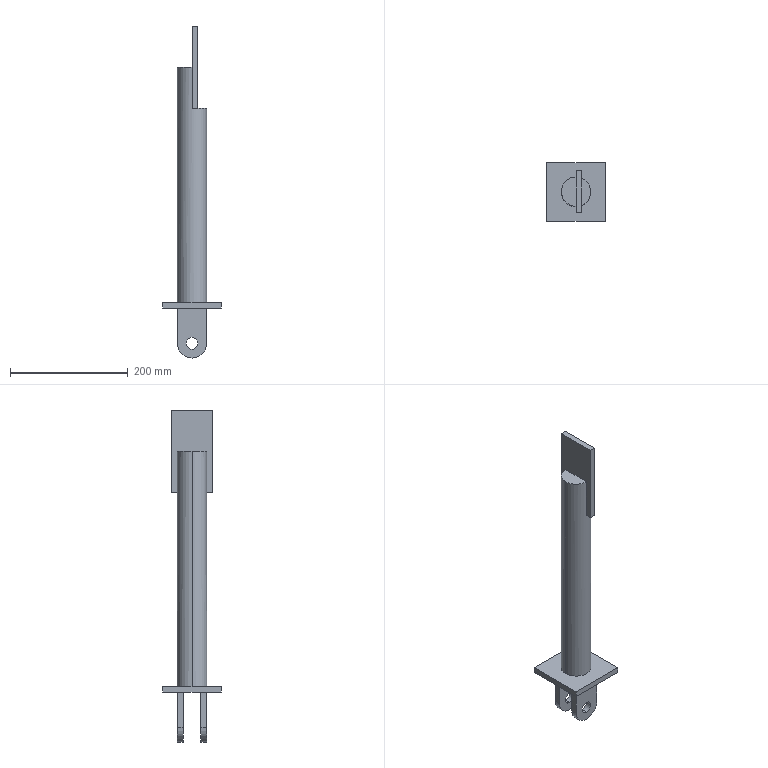Part | SolidWorks | features ICE 5, Extrusion 1 | 1 solid | 33 faces | box 100 x 100 x 565 mm | volume 988028 mm3 | plane 23 | cylinder 10 | commonest cylinder face diameters 50 x6 20 x4
STEP:
#1=CARTESIAN_POINT('',(25.,0.,335.));
#2=VERTEX_POINT('',#1);
#3=CARTESIAN_POINT('',(10.,22.913,335.));
#4=VERTEX_POINT('',#3);
#5=CARTESIAN_POINT('',(0.,0.,335.));
#6=DIRECTION('',(0.,0.,1.));
#7=DIRECTION('',(1.,0.,0.));
#8=AXIS2_PLACEMENT_3D('',#5,#6,#7);
#9=CIRCLE('',#8,25.);
#10=EDGE_CURVE('',#2,#4,#9,.T.);
#11=ORIENTED_EDGE('',*,*,#10,.F.);
#12=CARTESIAN_POINT('',(25.,0.,5.));
#13=VERTEX_POINT('',#12);
#14=CARTESIAN_POINT('',(25.,0.,405.));
#15=DIRECTION('',(0.,0.,-1.));
#16=VECTOR('',#15,1000.);
#17=LINE('',#14,#16);
#18=EDGE_CURVE('',#2,#13,#17,.T.);
#19=ORIENTED_EDGE('',*,*,#18,.T.);
#20=CARTESIAN_POINT('',(-25.,0.,5.));
#21=VERTEX_POINT('',#20);
#22=CARTESIAN_POINT('',(0.,0.,5.));
#23=DIRECTION('',(0.,0.,1.));
#24=DIRECTION('',(1.,0.,0.));
#25=AXIS2_PLACEMENT_3D('',#22,#23,#24);
#26=CIRCLE('',#25,25.);
#27=EDGE_CURVE('',#13,#21,#26,.T.);
#28=ORIENTED_EDGE('',*,*,#27,.T.);
#29=CARTESIAN_POINT('',(-25.,0.,405.));
#30=VERTEX_POINT('',#29);
#31=CARTESIAN_POINT('',(-25.,0.,405.));
#32=DIRECTION('',(0.,0.,-1.));
#33=VECTOR('',#32,1000.);
#34=LINE('',#31,#33);
#35=EDGE_CURVE('',#30,#21,#34,.T.);
#36=ORIENTED_EDGE('',*,*,#35,.F.);
#37=CARTESIAN_POINT('',(0.,25.,405.));
#38=VERTEX_POINT('',#37);
#39=CARTESIAN_POINT('',(0.,0.,405.));
#40=DIRECTION('',(0.,0.,1.));
#41=DIRECTION('',(1.,0.,0.));
#42=AXIS2_PLACEMENT_3D('',#39,#40,#41);
#43=CIRCLE('',#42,25.);
#44=EDGE_CURVE('',#38,#30,#43,.T.);
#45=ORIENTED_EDGE('',*,*,#44,.F.);
#46=CARTESIAN_POINT('',(0.,25.,335.));
#47=VERTEX_POINT('',#46);
#48=CARTESIAN_POINT('',(0.,25.,335.));
#49=DIRECTION('',(0.,0.,1.));
#50=VECTOR('',#49,1000.);
#51=LINE('',#48,#50);
#52=EDGE_CURVE('',#47,#38,#51,.T.);
#53=ORIENTED_EDGE('',*,*,#52,.F.);
#54=CARTESIAN_POINT('',(0.,0.,335.));
#55=DIRECTION('',(0.,0.,1.));
#56=DIRECTION('',(1.,0.,0.));
#57=AXIS2_PLACEMENT_3D('',#54,#55,#56);
#58=CIRCLE('',#57,25.);
#59=EDGE_CURVE('',#4,#47,#58,.T.);
#60=ORIENTED_EDGE('',*,*,#59,.F.);
#61=EDGE_LOOP('',(#11,#19,#28,#36,#45,#53,#60));
#62=FACE_OUTER_BOUND('',#61,.T.);
#63=CARTESIAN_POINT('',(0.,0.,405.));
#64=DIRECTION('',(0.,0.,-1.));
#65=DIRECTION('',(-1.,0.,0.));
#66=AXIS2_PLACEMENT_3D('',#63,#64,#65);
#67=CYLINDRICAL_SURFACE('',#66,25.);
#68=ADVANCED_FACE('',(#62),#67,.T.);
#69=CARTESIAN_POINT('',(0.,25.,-75.));
#70=VERTEX_POINT('',#69);
#71=CARTESIAN_POINT('',(0.,25.,-55.));
#72=VERTEX_POINT('',#71);
#73=CARTESIAN_POINT('',(0.,25.,-65.));
#74=DIRECTION('',(0.,1.,0.));
#75=DIRECTION('',(0.,0.,1.));
#76=AXIS2_PLACEMENT_3D('',#73,#74,#75);
#77=CIRCLE('',#76,10.);
#78=EDGE_CURVE('',#70,#72,#77,.T.);
#79=ORIENTED_EDGE('',*,*,#78,.T.);
#80=CARTESIAN_POINT('',(0.,15.,-55.));
#81=VERTEX_POINT('',#80);
#82=CARTESIAN_POINT('',(0.,25.,-55.));
#83=DIRECTION('',(0.,-1.,0.));
#84=VECTOR('',#83,1000.);
#85=LINE('',#82,#84);
#86=EDGE_CURVE('',#72,#81,#85,.T.);
#87=ORIENTED_EDGE('',*,*,#86,.T.);
#88=CARTESIAN_POINT('',(0.,15.,-75.));
#89=VERTEX_POINT('',#88);
#90=CARTESIAN_POINT('',(0.,15.,-65.));
#91=DIRECTION('',(0.,-1.,0.));
#92=DIRECTION('',(0.,0.,-1.));
#93=AXIS2_PLACEMENT_3D('',#90,#91,#92);
#94=CIRCLE('',#93,10.);
#95=EDGE_CURVE('',#81,#89,#94,.T.);
#96=ORIENTED_EDGE('',*,*,#95,.T.);
#97=CARTESIAN_POINT('',(0.,25.,-75.));
#98=DIRECTION('',(0.,-1.,0.));
#99=VECTOR('',#98,1000.);
#100=LINE('',#97,#99);
#101=EDGE_CURVE('',#70,#89,#100,.T.);
#102=ORIENTED_EDGE('',*,*,#101,.F.);
#103=EDGE_LOOP('',(#79,#87,#96,#102));
#104=FACE_OUTER_BOUND('',#103,.T.);
#105=CARTESIAN_POINT('',(0.,25.,-65.));
#106=DIRECTION('',(0.,-1.,0.));
#107=DIRECTION('',(0.,0.,-1.));
#108=AXIS2_PLACEMENT_3D('',#105,#106,#107);
#109=CYLINDRICAL_SURFACE('',#108,10.);
#110=ADVANCED_FACE('',(#104),#109,.F.);
#111=CARTESIAN_POINT('',(0.,-15.,-75.));
#112=VERTEX_POINT('',#111);
#113=CARTESIAN_POINT('',(0.,-15.,-55.));
#114=VERTEX_POINT('',#113);
#115=CARTESIAN_POINT('',(0.,-15.,-65.));
#116=DIRECTION('',(0.,1.,0.));
#117=DIRECTION('',(-1.,0.,0.));
#118=AXIS2_PLACEMENT_3D('',#115,#116,#117);
#119=CIRCLE('',#118,10.);
#120=EDGE_CURVE('',#112,#114,#119,.T.);
#121=ORIENTED_EDGE('',*,*,#120,.T.);
#122=CARTESIAN_POINT('',(0.,-25.,-55.));
#123=VERTEX_POINT('',#122);
#124=CARTESIAN_POINT('',(0.,25.,-55.));
#125=DIRECTION('',(0.,-1.,0.));
#126=VECTOR('',#125,1000.);
#127=LINE('',#124,#126);
#128=EDGE_CURVE('',#114,#123,#127,.T.);
#129=ORIENTED_EDGE('',*,*,#128,.T.);
#130=CARTESIAN_POINT('',(0.,-25.,-75.));
#131=VERTEX_POINT('',#130);
#132=CARTESIAN_POINT('',(0.,-25.,-65.));
#133=DIRECTION('',(0.,1.,0.));
#134=DIRECTION('',(0.,0.,1.));
#135=AXIS2_PLACEMENT_3D('',#132,#133,#134);
#136=CIRCLE('',#135,10.);
#137=EDGE_CURVE('',#131,#123,#136,.T.);
#138=ORIENTED_EDGE('',*,*,#137,.F.);
#139=CARTESIAN_POINT('',(0.,25.,-75.));
#140=DIRECTION('',(0.,-1.,0.));
#141=VECTOR('',#140,1000.);
#142=LINE('',#139,#141);
#143=EDGE_CURVE('',#112,#131,#142,.T.);
#144=ORIENTED_EDGE('',*,*,#143,.F.);
#145=EDGE_LOOP('',(#121,#129,#138,#144));
#146=FACE_OUTER_BOUND('',#145,.T.);
#147=CARTESIAN_POINT('',(0.,25.,-65.));
#148=DIRECTION('',(0.,-1.,0.));
#149=DIRECTION('',(0.,0.,-1.));
#150=AXIS2_PLACEMENT_3D('',#147,#148,#149);
#151=CYLINDRICAL_SURFACE('',#150,10.);
#152=ADVANCED_FACE('',(#146),#151,.F.);
#153=CARTESIAN_POINT('',(0.,25.,-90.));
#154=VERTEX_POINT('',#153);
#155=CARTESIAN_POINT('',(-25.,25.,-65.));
#156=VERTEX_POINT('',#155);
#157=CARTESIAN_POINT('',(0.,25.,-65.));
#158=DIRECTION('',(0.,1.,0.));
#159=DIRECTION('',(0.,0.,1.));
#160=AXIS2_PLACEMENT_3D('',#157,#158,#159);
#161=CIRCLE('',#160,25.);
#162=EDGE_CURVE('',#154,#156,#161,.T.);
#163=ORIENTED_EDGE('',*,*,#162,.F.);
#164=CARTESIAN_POINT('',(0.,15.,-90.));
#165=VERTEX_POINT('',#164);
#166=CARTESIAN_POINT('',(0.,25.,-90.));
#167=DIRECTION('',(0.,-1.,0.));
#168=VECTOR('',#167,1000.);
#169=LINE('',#166,#168);
#170=EDGE_CURVE('',#154,#165,#169,.T.);
#171=ORIENTED_EDGE('',*,*,#170,.T.);
#172=CARTESIAN_POINT('',(-25.,15.,-65.));
#173=VERTEX_POINT('',#172);
#174=CARTESIAN_POINT('',(0.,15.,-65.));
#175=DIRECTION('',(0.,-1.,0.));
#176=DIRECTION('',(0.,0.,-1.));
#177=AXIS2_PLACEMENT_3D('',#174,#175,#176);
#178=CIRCLE('',#177,25.);
#179=EDGE_CURVE('',#173,#165,#178,.T.);
#180=ORIENTED_EDGE('',*,*,#179,.F.);
#181=CARTESIAN_POINT('',(-25.,25.,-65.));
#182=DIRECTION('',(0.,-1.,0.));
#183=VECTOR('',#182,1000.);
#184=LINE('',#181,#183);
#185=EDGE_CURVE('',#156,#173,#184,.T.);
#186=ORIENTED_EDGE('',*,*,#185,.F.);
#187=EDGE_LOOP('',(#163,#171,#180,#186));
#188=FACE_OUTER_BOUND('',#187,.T.);
#189=CARTESIAN_POINT('',(0.,25.,-65.));
#190=DIRECTION('',(0.,-1.,0.));
#191=DIRECTION('',(0.,0.,-1.));
#192=AXIS2_PLACEMENT_3D('',#189,#190,#191);
#193=CYLINDRICAL_SURFACE('',#192,25.);
#194=ADVANCED_FACE('',(#188),#193,.T.);
#195=CARTESIAN_POINT('',(0.,-15.,-90.));
#196=VERTEX_POINT('',#195);
#197=CARTESIAN_POINT('',(-25.,-15.,-65.));
#198=VERTEX_POINT('',#197);
#199=CARTESIAN_POINT('',(0.,-15.,-65.));
#200=DIRECTION('',(0.,1.,0.));
#201=DIRECTION('',(-1.,0.,0.));
#202=AXIS2_PLACEMENT_3D('',#199,#200,#201);
#203=CIRCLE('',#202,25.);
#204=EDGE_CURVE('',#196,#198,#203,.T.);
#205=ORIENTED_EDGE('',*,*,#204,.F.);
#206=CARTESIAN_POINT('',(0.,-25.,-90.));
#207=VERTEX_POINT('',#206);
#208=CARTESIAN_POINT('',(0.,25.,-90.));
#209=DIRECTION('',(0.,-1.,0.));
#210=VECTOR('',#209,1000.);
#211=LINE('',#208,#210);
#212=EDGE_CURVE('',#196,#207,#211,.T.);
#213=ORIENTED_EDGE('',*,*,#212,.T.);
#214=CARTESIAN_POINT('',(-25.,-25.,-65.));
#215=VERTEX_POINT('',#214);
#216=CARTESIAN_POINT('',(0.,-25.,-65.));
#217=DIRECTION('',(0.,1.,0.));
#218=DIRECTION('',(0.,0.,1.));
#219=AXIS2_PLACEMENT_3D('',#216,#217,#218);
#220=CIRCLE('',#219,25.);
#221=EDGE_CURVE('',#207,#215,#220,.T.);
#222=ORIENTED_EDGE('',*,*,#221,.T.);
#223=CARTESIAN_POINT('',(-25.,25.,-65.));
#224=DIRECTION('',(0.,-1.,0.));
#225=VECTOR('',#224,1000.);
#226=LINE('',#223,#225);
#227=EDGE_CURVE('',#198,#215,#226,.T.);
#228=ORIENTED_EDGE('',*,*,#227,.F.);
#229=EDGE_LOOP('',(#205,#213,#222,#228));
#230=FACE_OUTER_BOUND('',#229,.T.);
#231=CARTESIAN_POINT('',(0.,25.,-65.));
#232=DIRECTION('',(0.,-1.,0.));
#233=DIRECTION('',(0.,0.,-1.));
#234=AXIS2_PLACEMENT_3D('',#231,#232,#233);
#235=CYLINDRICAL_SURFACE('',#234,25.);
#236=ADVANCED_FACE('',(#230),#235,.T.);
#237=CARTESIAN_POINT('',(10.,-22.913,335.));
#238=VERTEX_POINT('',#237);
#239=CARTESIAN_POINT('',(0.,0.,335.));
#240=DIRECTION('',(0.,0.,1.));
#241=DIRECTION('',(1.,0.,0.));
#242=AXIS2_PLACEMENT_3D('',#239,#240,#241);
#243=CIRCLE('',#242,25.);
#244=EDGE_CURVE('',#238,#2,#243,.T.);
#245=ORIENTED_EDGE('',*,*,#244,.T.);
#246=ORIENTED_EDGE('',*,*,#10,.T.);
#247=CARTESIAN_POINT('',(10.,0.,335.));
#248=DIRECTION('',(0.,-1.,0.));
#249=VECTOR('',#248,1000.);
#250=LINE('',#247,#249);
#251=EDGE_CURVE('',#4,#238,#250,.T.);
#252=ORIENTED_EDGE('',*,*,#251,.T.);
#253=EDGE_LOOP('',(#245,#246,#252));
#254=FACE_OUTER_BOUND('',#253,.T.);
#255=CARTESIAN_POINT('',(0.,0.,335.));
#256=DIRECTION('',(0.,0.,1.));
#257=DIRECTION('',(1.,0.,0.));
#258=AXIS2_PLACEMENT_3D('',#255,#256,#257);
#259=PLANE('',#258);
#260=ADVANCED_FACE('',(#254),#259,.T.);
#261=CARTESIAN_POINT('',(-25.,-15.,-5.));
#262=VERTEX_POINT('',#261);
#263=CARTESIAN_POINT('',(-25.,-15.,-135.));
#264=DIRECTION('',(0.,0.,1.));
#265=VECTOR('',#264,1000.);
#266=LINE('',#263,#265);
#267=EDGE_CURVE('',#198,#262,#266,.T.);
#268=ORIENTED_EDGE('',*,*,#267,.F.);
#269=ORIENTED_EDGE('',*,*,#227,.T.);
#270=CARTESIAN_POINT('',(-25.,-25.,-5.));
#271=VERTEX_POINT('',#270);
#272=CARTESIAN_POINT('',(-25.,-25.,-5.));
#273=DIRECTION('',(0.,0.,1.));
#274=VECTOR('',#273,1000.);
#275=LINE('',#272,#274);
#276=EDGE_CURVE('',#215,#271,#275,.T.);
#277=ORIENTED_EDGE('',*,*,#276,.T.);
#278=CARTESIAN_POINT('',(-25.,25.,-5.));
#279=DIRECTION('',(0.,-1.,0.));
#280=VECTOR('',#279,1000.);
#281=LINE('',#278,#280);
#282=EDGE_CURVE('',#262,#271,#281,.T.);
#283=ORIENTED_EDGE('',*,*,#282,.F.);
#284=EDGE_LOOP('',(#268,#269,#277,#283));
#285=FACE_OUTER_BOUND('',#284,.T.);
#286=CARTESIAN_POINT('',(-25.,25.,-5.));
#287=DIRECTION('',(1.,0.,0.));
#288=DIRECTION('',(0.,0.,-1.));
#289=AXIS2_PLACEMENT_3D('',#286,#287,#288);
#290=PLANE('',#289);
#291=ADVANCED_FACE('',(#285),#290,.F.);
#292=CARTESIAN_POINT('',(-25.,15.,-5.));
#293=VERTEX_POINT('',#292);
#294=CARTESIAN_POINT('',(-25.,15.,-135.));
#295=DIRECTION('',(0.,0.,1.));
#296=VECTOR('',#295,1000.);
#297=LINE('',#294,#296);
#298=EDGE_CURVE('',#173,#293,#297,.T.);
#299=ORIENTED_EDGE('',*,*,#298,.T.);
#300=CARTESIAN_POINT('',(-25.,25.,-5.));
#301=VERTEX_POINT('',#300);
#302=CARTESIAN_POINT('',(-25.,25.,-5.));
#303=DIRECTION('',(0.,-1.,0.));
#304=VECTOR('',#303,1000.);
#305=LINE('',#302,#304);
#306=EDGE_CURVE('',#301,#293,#305,.T.);
#307=ORIENTED_EDGE('',*,*,#306,.F.);
#308=CARTESIAN_POINT('',(-25.,25.,-5.));
#309=DIRECTION('',(0.,0.,1.));
#310=VECTOR('',#309,1000.);
#311=LINE('',#308,#310);
#312=EDGE_CURVE('',#156,#301,#311,.T.);
#313=ORIENTED_EDGE('',*,*,#312,.F.);
#314=ORIENTED_EDGE('',*,*,#185,.T.);
#315=EDGE_LOOP('',(#299,#307,#313,#314));
#316=FACE_OUTER_BOUND('',#315,.T.);
#317=CARTESIAN_POINT('',(-25.,25.,-5.));
#318=DIRECTION('',(1.,0.,0.));
#319=DIRECTION('',(0.,0.,-1.));
#320=AXIS2_PLACEMENT_3D('',#317,#318,#319);
#321=PLANE('',#320);
#322=ADVANCED_FACE('',(#316),#321,.F.);
#323=CARTESIAN_POINT('',(25.,-15.,-65.));
#324=VERTEX_POINT('',#323);
#325=CARTESIAN_POINT('',(25.,-15.,-5.));
#326=VERTEX_POINT('',#325);
#327=CARTESIAN_POINT('',(25.,-15.,-135.));
#328=DIRECTION('',(0.,0.,1.));
#329=VECTOR('',#328,1000.);
#330=LINE('',#327,#329);
#331=EDGE_CURVE('',#324,#326,#330,.T.);
#332=ORIENTED_EDGE('',*,*,#331,.T.);
#333=CARTESIAN_POINT('',(25.,-25.,-5.));
#334=VERTEX_POINT('',#333);
#335=CARTESIAN_POINT('',(25.,25.,-5.));
#336=DIRECTION('',(0.,-1.,0.));
#337=VECTOR('',#336,1000.);
#338=LINE('',#335,#337);
#339=EDGE_CURVE('',#326,#334,#338,.T.);
#340=ORIENTED_EDGE('',*,*,#339,.T.);
#341=CARTESIAN_POINT('',(25.,-25.,-65.));
#342=VERTEX_POINT('',#341);
#343=CARTESIAN_POINT('',(25.,-25.,-5.));
#344=DIRECTION('',(0.,0.,-1.));
#345=VECTOR('',#344,1000.);
#346=LINE('',#343,#345);
#347=EDGE_CURVE('',#334,#342,#346,.T.);
#348=ORIENTED_EDGE('',*,*,#347,.T.);
#349=CARTESIAN_POINT('',(25.,25.,-65.));
#350=DIRECTION('',(0.,-1.,0.));
#351=VECTOR('',#350,1000.);
#352=LINE('',#349,#351);
#353=EDGE_CURVE('',#324,#342,#352,.T.);
#354=ORIENTED_EDGE('',*,*,#353,.F.);
#355=EDGE_LOOP('',(#332,#340,#348,#354));
#356=FACE_OUTER_BOUND('',#355,.T.);
#357=CARTESIAN_POINT('',(25.,25.,-5.));
#358=DIRECTION('',(-1.,0.,0.));
#359=DIRECTION('',(0.,0.,1.));
#360=AXIS2_PLACEMENT_3D('',#357,#358,#359);
#361=PLANE('',#360);
#362=ADVANCED_FACE('',(#356),#361,.F.);
#363=CARTESIAN_POINT('',(25.,15.,-65.));
#364=VERTEX_POINT('',#363);
#365=CARTESIAN_POINT('',(25.,15.,-5.));
#366=VERTEX_POINT('',#365);
#367=CARTESIAN_POINT('',(25.,15.,-135.));
#368=DIRECTION('',(0.,0.,1.));
#369=VECTOR('',#368,1000.);
#370=LINE('',#367,#369);
#371=EDGE_CURVE('',#364,#366,#370,.T.);
#372=ORIENTED_EDGE('',*,*,#371,.F.);
#373=CARTESIAN_POINT('',(25.,25.,-65.));
#374=VERTEX_POINT('',#373);
#375=CARTESIAN_POINT('',(25.,25.,-65.));
#376=DIRECTION('',(0.,-1.,0.));
#377=VECTOR('',#376,1000.);
#378=LINE('',#375,#377);
#379=EDGE_CURVE('',#374,#364,#378,.T.);
#380=ORIENTED_EDGE('',*,*,#379,.F.);
#381=CARTESIAN_POINT('',(25.,25.,-5.));
#382=VERTEX_POINT('',#381);
#383=CARTESIAN_POINT('',(25.,25.,-5.));
#384=DIRECTION('',(0.,0.,-1.));
#385=VECTOR('',#384,1000.);
#386=LINE('',#383,#385);
#387=EDGE_CURVE('',#382,#374,#386,.T.);
#388=ORIENTED_EDGE('',*,*,#387,.F.);
#389=CARTESIAN_POINT('',(25.,25.,-5.));
#390=DIRECTION('',(0.,-1.,0.));
#391=VECTOR('',#390,1000.);
#392=LINE('',#389,#391);
#393=EDGE_CURVE('',#382,#366,#392,.T.);
#394=ORIENTED_EDGE('',*,*,#393,.T.);
#395=EDGE_LOOP('',(#372,#380,#388,#394));
#396=FACE_OUTER_BOUND('',#395,.T.);
#397=CARTESIAN_POINT('',(25.,25.,-5.));
#398=DIRECTION('',(-1.,0.,0.));
#399=DIRECTION('',(0.,0.,1.));
#400=AXIS2_PLACEMENT_3D('',#397,#398,#399);
#401=PLANE('',#400);
#402=ADVANCED_FACE('',(#396),#401,.F.);
#403=ORIENTED_EDGE('',*,*,#212,.F.);
#404=CARTESIAN_POINT('',(0.,-15.,-65.));
#405=DIRECTION('',(0.,1.,0.));
#406=DIRECTION('',(-1.,0.,0.));
#407=AXIS2_PLACEMENT_3D('',#404,#405,#406);
#408=CIRCLE('',#407,25.);
#409=EDGE_CURVE('',#324,#196,#408,.T.);
#410=ORIENTED_EDGE('',*,*,#409,.F.);
#411=ORIENTED_EDGE('',*,*,#353,.T.);
#412=CARTESIAN_POINT('',(0.,-25.,-65.));
#413=DIRECTION('',(0.,1.,0.));
#414=DIRECTION('',(0.,0.,1.));
#415=AXIS2_PLACEMENT_3D('',#412,#413,#414);
#416=CIRCLE('',#415,25.);
#417=EDGE_CURVE('',#342,#207,#416,.T.);
#418=ORIENTED_EDGE('',*,*,#417,.T.);
#419=EDGE_LOOP('',(#403,#410,#411,#418));
#420=FACE_OUTER_BOUND('',#419,.T.);
#421=CARTESIAN_POINT('',(0.,25.,-65.));
#422=DIRECTION('',(0.,-1.,0.));
#423=DIRECTION('',(0.,0.,-1.));
#424=AXIS2_PLACEMENT_3D('',#421,#422,#423);
#425=CYLINDRICAL_SURFACE('',#424,25.);
#426=ADVANCED_FACE('',(#420),#425,.T.);
#427=ORIENTED_EDGE('',*,*,#170,.F.);
#428=CARTESIAN_POINT('',(0.,25.,-65.));
#429=DIRECTION('',(0.,1.,0.));
#430=DIRECTION('',(0.,0.,1.));
#431=AXIS2_PLACEMENT_3D('',#428,#429,#430);
#432=CIRCLE('',#431,25.);
#433=EDGE_CURVE('',#374,#154,#432,.T.);
#434=ORIENTED_EDGE('',*,*,#433,.F.);
#435=ORIENTED_EDGE('',*,*,#379,.T.);
#436=CARTESIAN_POINT('',(0.,15.,-65.));
#437=DIRECTION('',(0.,-1.,0.));
#438=DIRECTION('',(0.,0.,-1.));
#439=AXIS2_PLACEMENT_3D('',#436,#437,#438);
#440=CIRCLE('',#439,25.);
#441=EDGE_CURVE('',#165,#364,#440,.T.);
#442=ORIENTED_EDGE('',*,*,#441,.F.);
#443=EDGE_LOOP('',(#427,#434,#435,#442));
#444=FACE_OUTER_BOUND('',#443,.T.);
#445=CARTESIAN_POINT('',(0.,25.,-65.));
#446=DIRECTION('',(0.,-1.,0.));
#447=DIRECTION('',(0.,0.,-1.));
#448=AXIS2_PLACEMENT_3D('',#445,#446,#447);
#449=CYLINDRICAL_SURFACE('',#448,25.);
#450=ADVANCED_FACE('',(#444),#449,.T.);
#451=ORIENTED_EDGE('',*,*,#128,.F.);
#452=CARTESIAN_POINT('',(0.,-15.,-65.));
#453=DIRECTION('',(0.,1.,0.));
#454=DIRECTION('',(-1.,0.,0.));
#455=AXIS2_PLACEMENT_3D('',#452,#453,#454);
#456=CIRCLE('',#455,10.);
#457=EDGE_CURVE('',#114,#112,#456,.T.);
#458=ORIENTED_EDGE('',*,*,#457,.T.);
#459=ORIENTED_EDGE('',*,*,#143,.T.);
#460=CARTESIAN_POINT('',(0.,-25.,-65.));
#461=DIRECTION('',(0.,1.,0.));
#462=DIRECTION('',(0.,0.,1.));
#463=AXIS2_PLACEMENT_3D('',#460,#461,#462);
#464=CIRCLE('',#463,10.);
#465=EDGE_CURVE('',#123,#131,#464,.T.);
#466=ORIENTED_EDGE('',*,*,#465,.F.);
#467=EDGE_LOOP('',(#451,#458,#459,#466));
#468=FACE_OUTER_BOUND('',#467,.T.);
#469=CARTESIAN_POINT('',(0.,25.,-65.));
#470=DIRECTION('',(0.,-1.,0.));
#471=DIRECTION('',(0.,0.,-1.));
#472=AXIS2_PLACEMENT_3D('',#469,#470,#471);
#473=CYLINDRICAL_SURFACE('',#472,10.);
#474=ADVANCED_FACE('',(#468),#473,.F.);
#475=ORIENTED_EDGE('',*,*,#86,.F.);
#476=CARTESIAN_POINT('',(0.,25.,-65.));
#477=DIRECTION('',(0.,1.,0.));
#478=DIRECTION('',(0.,0.,1.));
#479=AXIS2_PLACEMENT_3D('',#476,#477,#478);
#480=CIRCLE('',#479,10.);
#481=EDGE_CURVE('',#72,#70,#480,.T.);
#482=ORIENTED_EDGE('',*,*,#481,.T.);
#483=ORIENTED_EDGE('',*,*,#101,.T.);
#484=CARTESIAN_POINT('',(0.,15.,-65.));
#485=DIRECTION('',(0.,-1.,0.));
#486=DIRECTION('',(0.,0.,-1.));
#487=AXIS2_PLACEMENT_3D('',#484,#485,#486);
#488=CIRCLE('',#487,10.);
#489=EDGE_CURVE('',#89,#81,#488,.T.);
#490=ORIENTED_EDGE('',*,*,#489,.T.);
#491=EDGE_LOOP('',(#475,#482,#483,#490));
#492=FACE_OUTER_BOUND('',#491,.T.);
#493=CARTESIAN_POINT('',(0.,25.,-65.));
#494=DIRECTION('',(0.,-1.,0.));
#495=DIRECTION('',(0.,0.,-1.));
#496=AXIS2_PLACEMENT_3D('',#493,#494,#495);
#497=CYLINDRICAL_SURFACE('',#496,10.);
#498=ADVANCED_FACE('',(#492),#497,.F.);
#499=CARTESIAN_POINT('',(50.,-50.,-5.));
#500=VERTEX_POINT('',#499);
#501=CARTESIAN_POINT('',(50.,50.,-5.));
#502=VERTEX_POINT('',#501);
#503=CARTESIAN_POINT('',(50.,50.,-5.));
#504=DIRECTION('',(0.,1.,0.));
#505=VECTOR('',#504,1000.);
#506=LINE('',#503,#505);
#507=EDGE_CURVE('',#500,#502,#506,.T.);
#508=ORIENTED_EDGE('',*,*,#507,.T.);
#509=CARTESIAN_POINT('',(50.,50.,5.));
#510=VERTEX_POINT('',#509);
#511=CARTESIAN_POINT('',(50.,50.,5.));
#512=DIRECTION('',(0.,0.,-1.));
#513=VECTOR('',#512,1000.);
#514=LINE('',#511,#513);
#515=EDGE_CURVE('',#510,#502,#514,.T.);
#516=ORIENTED_EDGE('',*,*,#515,.F.);
#517=CARTESIAN_POINT('',(50.,-50.,5.));
#518=VERTEX_POINT('',#517);
#519=CARTESIAN_POINT('',(50.,50.,5.));
#520=DIRECTION('',(0.,1.,0.));
#521=VECTOR('',#520,1000.);
#522=LINE('',#519,#521);
#523=EDGE_CURVE('',#518,#510,#522,.T.);
#524=ORIENTED_EDGE('',*,*,#523,.F.);
#525=CARTESIAN_POINT('',(50.,-50.,5.));
#526=DIRECTION('',(0.,0.,-1.));
#527=VECTOR('',#526,1000.);
#528=LINE('',#525,#527);
#529=EDGE_CURVE('',#518,#500,#528,.T.);
#530=ORIENTED_EDGE('',*,*,#529,.T.);
#531=EDGE_LOOP('',(#508,#516,#524,#530));
#532=FACE_OUTER_BOUND('',#531,.T.);
#533=CARTESIAN_POINT('',(50.,50.,5.));
#534=DIRECTION('',(-1.,0.,0.));
#535=DIRECTION('',(0.,-1.,0.));
#536=AXIS2_PLACEMENT_3D('',#533,#534,#535);
#537=PLANE('',#536);
#538=ADVANCED_FACE('',(#532),#537,.F.);
#539=CARTESIAN_POINT('',(-50.,50.,-5.));
#540=VERTEX_POINT('',#539);
#541=CARTESIAN_POINT('',(-50.,50.,-5.));
#542=DIRECTION('',(-1.,0.,0.));
#543=VECTOR('',#542,1000.);
#544=LINE('',#541,#543);
#545=EDGE_CURVE('',#502,#540,#544,.T.);
#546=ORIENTED_EDGE('',*,*,#545,.T.);
#547=CARTESIAN_POINT('',(-50.,50.,5.));
#548=VERTEX_POINT('',#547);
#549=CARTESIAN_POINT('',(-50.,50.,5.));
#550=DIRECTION('',(0.,0.,-1.));
#551=VECTOR('',#550,1000.);
#552=LINE('',#549,#551);
#553=EDGE_CURVE('',#548,#540,#552,.T.);
#554=ORIENTED_EDGE('',*,*,#553,.F.);
#555=CARTESIAN_POINT('',(-50.,50.,5.));
#556=DIRECTION('',(-1.,0.,0.));
#557=VECTOR('',#556,1000.);
#558=LINE('',#555,#557);
#559=EDGE_CURVE('',#510,#548,#558,.T.);
#560=ORIENTED_EDGE('',*,*,#559,.F.);
#561=ORIENTED_EDGE('',*,*,#515,.T.);
#562=EDGE_LOOP('',(#546,#554,#560,#561));
#563=FACE_OUTER_BOUND('',#562,.T.);
#564=CARTESIAN_POINT('',(-50.,50.,5.));
#565=DIRECTION('',(0.,-1.,0.));
#566=DIRECTION('',(0.,0.,-1.));
#567=AXIS2_PLACEMENT_3D('',#564,#565,#566);
#568=PLANE('',#567);
#569=ADVANCED_FACE('',(#563),#568,.F.);
#570=CARTESIAN_POINT('',(-50.,-50.,-5.));
#571=VERTEX_POINT('',#570);
#572=CARTESIAN_POINT('',(-50.,50.,-5.));
#573=DIRECTION('',(0.,-1.,0.));
#574=VECTOR('',#573,1000.);
#575=LINE('',#572,#574);
#576=EDGE_CURVE('',#540,#571,#575,.T.);
#577=ORIENTED_EDGE('',*,*,#576,.T.);
#578=CARTESIAN_POINT('',(-50.,-50.,5.));
#579=VERTEX_POINT('',#578);
#580=CARTESIAN_POINT('',(-50.,-50.,5.));
#581=DIRECTION('',(0.,0.,-1.));
#582=VECTOR('',#581,1000.);
#583=LINE('',#580,#582);
#584=EDGE_CURVE('',#579,#571,#583,.T.);
#585=ORIENTED_EDGE('',*,*,#584,.F.);
#586=CARTESIAN_POINT('',(-50.,50.,5.));
#587=DIRECTION('',(0.,-1.,0.));
#588=VECTOR('',#587,1000.);
#589=LINE('',#586,#588);
#590=EDGE_CURVE('',#548,#579,#589,.T.);
#591=ORIENTED_EDGE('',*,*,#590,.F.);
#592=ORIENTED_EDGE('',*,*,#553,.T.);
#593=EDGE_LOOP('',(#577,#585,#591,#592));
#594=FACE_OUTER_BOUND('',#593,.T.);
#595=CARTESIAN_POINT('',(-50.,50.,5.));
#596=DIRECTION('',(1.,0.,0.));
#597=DIRECTION('',(0.,1.,0.));
#598=AXIS2_PLACEMENT_3D('',#595,#596,#597);
#599=PLANE('',#598);
#600=ADVANCED_FACE('',(#594),#599,.F.);
#601=CARTESIAN_POINT('',(-50.,-50.,-5.));
#602=DIRECTION('',(1.,0.,0.));
#603=VECTOR('',#602,1000.);
#604=LINE('',#601,#603);
#605=EDGE_CURVE('',#571,#500,#604,.T.);
#606=ORIENTED_EDGE('',*,*,#605,.T.);
#607=ORIENTED_EDGE('',*,*,#529,.F.);
#608=CARTESIAN_POINT('',(-50.,-50.,5.));
#609=DIRECTION('',(1.,0.,0.));
#610=VECTOR('',#609,1000.);
#611=LINE('',#608,#610);
#612=EDGE_CURVE('',#579,#518,#611,.T.);
#613=ORIENTED_EDGE('',*,*,#612,.F.);
#614=ORIENTED_EDGE('',*,*,#584,.T.);
#615=EDGE_LOOP('',(#606,#607,#613,#614));
#616=FACE_OUTER_BOUND('',#615,.T.);
#617=CARTESIAN_POINT('',(-50.,-50.,5.));
#618=DIRECTION('',(0.,1.,0.));
#619=DIRECTION('',(0.,0.,1.));
#620=AXIS2_PLACEMENT_3D('',#617,#618,#619);
#621=PLANE('',#620);
#622=ADVANCED_FACE('',(#616),#621,.F.);
#623=CARTESIAN_POINT('',(0.,0.,5.));
#624=DIRECTION('',(0.,0.,1.));
#625=DIRECTION('',(1.,0.,0.));
#626=AXIS2_PLACEMENT_3D('',#623,#624,#625);
#627=CIRCLE('',#626,25.);
#628=EDGE_CURVE('',#21,#13,#627,.T.);
#629=ORIENTED_EDGE('',*,*,#628,.F.);
#630=ORIENTED_EDGE('',*,*,#27,.F.);
#631=EDGE_LOOP('',(#629,#630));
#632=FACE_BOUND('',#631,.T.);
#633=ORIENTED_EDGE('',*,*,#523,.T.);
#634=ORIENTED_EDGE('',*,*,#559,.T.);
#635=ORIENTED_EDGE('',*,*,#590,.T.);
#636=ORIENTED_EDGE('',*,*,#612,.T.);
#637=EDGE_LOOP('',(#633,#634,#635,#636));
#638=FACE_OUTER_BOUND('',#637,.T.);
#639=CARTESIAN_POINT('',(0.,0.,5.));
#640=DIRECTION('',(0.,0.,1.));
#641=DIRECTION('',(1.,0.,0.));
#642=AXIS2_PLACEMENT_3D('',#639,#640,#641);
#643=PLANE('',#642);
#644=ADVANCED_FACE('',(#632,#638),#643,.T.);
#645=ORIENTED_EDGE('',*,*,#306,.T.);
#646=CARTESIAN_POINT('',(25.,15.,-5.));
#647=DIRECTION('',(1.,0.,0.));
#648=VECTOR('',#647,1000.);
#649=LINE('',#646,#648);
#650=EDGE_CURVE('',#293,#366,#649,.T.);
#651=ORIENTED_EDGE('',*,*,#650,.T.);
#652=ORIENTED_EDGE('',*,*,#393,.F.);
#653=CARTESIAN_POINT('',(-25.,25.,-5.));
#654=DIRECTION('',(1.,0.,0.));
#655=VECTOR('',#654,1000.);
#656=LINE('',#653,#655);
#657=EDGE_CURVE('',#301,#382,#656,.T.);
#658=ORIENTED_EDGE('',*,*,#657,.F.);
#659=EDGE_LOOP('',(#645,#651,#652,#658));
#660=FACE_BOUND('',#659,.T.);
#661=CARTESIAN_POINT('',(25.,-15.,-5.));
#662=DIRECTION('',(-1.,0.,0.));
#663=VECTOR('',#662,1000.);
#664=LINE('',#661,#663);
#665=EDGE_CURVE('',#326,#262,#664,.T.);
#666=ORIENTED_EDGE('',*,*,#665,.T.);
#667=ORIENTED_EDGE('',*,*,#282,.T.);
#668=CARTESIAN_POINT('',(-25.,-25.,-5.));
#669=DIRECTION('',(1.,0.,0.));
#670=VECTOR('',#669,1000.);
#671=LINE('',#668,#670);
#672=EDGE_CURVE('',#271,#334,#671,.T.);
#673=ORIENTED_EDGE('',*,*,#672,.T.);
#674=ORIENTED_EDGE('',*,*,#339,.F.);
#675=EDGE_LOOP('',(#666,#667,#673,#674));
#676=FACE_BOUND('',#675,.T.);
#677=ORIENTED_EDGE('',*,*,#507,.F.);
#678=ORIENTED_EDGE('',*,*,#605,.F.);
#679=ORIENTED_EDGE('',*,*,#576,.F.);
#680=ORIENTED_EDGE('',*,*,#545,.F.);
#681=EDGE_LOOP('',(#677,#678,#679,#680));
#682=FACE_OUTER_BOUND('',#681,.T.);
#683=CARTESIAN_POINT('',(0.,0.,-5.));
#684=DIRECTION('',(0.,0.,1.));
#685=DIRECTION('',(1.,0.,0.));
#686=AXIS2_PLACEMENT_3D('',#683,#684,#685);
#687=PLANE('',#686);
#688=ADVANCED_FACE('',(#660,#676,#682),#687,.F.);
#689=ORIENTED_EDGE('',*,*,#312,.T.);
#690=ORIENTED_EDGE('',*,*,#657,.T.);
#691=ORIENTED_EDGE('',*,*,#387,.T.);
#692=ORIENTED_EDGE('',*,*,#433,.T.);
#693=ORIENTED_EDGE('',*,*,#162,.T.);
#694=EDGE_LOOP('',(#689,#690,#691,#692,#693));
#695=FACE_OUTER_BOUND('',#694,.T.);
#696=ORIENTED_EDGE('',*,*,#78,.F.);
#697=ORIENTED_EDGE('',*,*,#481,.F.);
#698=EDGE_LOOP('',(#696,#697));
#699=FACE_BOUND('',#698,.T.);
#700=CARTESIAN_POINT('',(0.,25.,-65.));
#701=DIRECTION('',(0.,1.,0.));
#702=DIRECTION('',(0.,0.,1.));
#703=AXIS2_PLACEMENT_3D('',#700,#701,#702);
#704=PLANE('',#703);
#705=ADVANCED_FACE('',(#695,#699),#704,.T.);
#706=ORIENTED_EDGE('',*,*,#276,.F.);
#707=ORIENTED_EDGE('',*,*,#221,.F.);
#708=ORIENTED_EDGE('',*,*,#417,.F.);
#709=ORIENTED_EDGE('',*,*,#347,.F.);
#710=ORIENTED_EDGE('',*,*,#672,.F.);
#711=EDGE_LOOP('',(#706,#707,#708,#709,#710));
#712=FACE_OUTER_BOUND('',#711,.T.);
#713=ORIENTED_EDGE('',*,*,#137,.T.);
#714=ORIENTED_EDGE('',*,*,#465,.T.);
#715=EDGE_LOOP('',(#713,#714));
#716=FACE_BOUND('',#715,.T.);
#717=CARTESIAN_POINT('',(0.,-25.,-65.));
#718=DIRECTION('',(0.,1.,0.));
#719=DIRECTION('',(0.,0.,1.));
#720=AXIS2_PLACEMENT_3D('',#717,#718,#719);
#721=PLANE('',#720);
#722=ADVANCED_FACE('',(#712,#716),#721,.F.);
#723=ORIENTED_EDGE('',*,*,#120,.F.);
#724=ORIENTED_EDGE('',*,*,#457,.F.);
#725=EDGE_LOOP('',(#723,#724));
#726=FACE_BOUND('',#725,.T.);
#727=ORIENTED_EDGE('',*,*,#409,.T.);
#728=ORIENTED_EDGE('',*,*,#204,.T.);
#729=ORIENTED_EDGE('',*,*,#267,.T.);
#730=ORIENTED_EDGE('',*,*,#665,.F.);
#731=ORIENTED_EDGE('',*,*,#331,.F.);
#732=EDGE_LOOP('',(#727,#728,#729,#730,#731));
#733=FACE_OUTER_BOUND('',#732,.T.);
#734=CARTESIAN_POINT('',(25.,-15.,-135.));
#735=DIRECTION('',(0.,1.,0.));
#736=DIRECTION('',(-1.,0.,0.));
#737=AXIS2_PLACEMENT_3D('',#734,#735,#736);
#738=PLANE('',#737);
#739=ADVANCED_FACE('',(#726,#733),#738,.T.);
#740=ORIENTED_EDGE('',*,*,#489,.F.);
#741=ORIENTED_EDGE('',*,*,#95,.F.);
#742=EDGE_LOOP('',(#740,#741));
#743=FACE_BOUND('',#742,.T.);
#744=ORIENTED_EDGE('',*,*,#179,.T.);
#745=ORIENTED_EDGE('',*,*,#441,.T.);
#746=ORIENTED_EDGE('',*,*,#371,.T.);
#747=ORIENTED_EDGE('',*,*,#650,.F.);
#748=ORIENTED_EDGE('',*,*,#298,.F.);
#749=EDGE_LOOP('',(#744,#745,#746,#747,#748));
#750=FACE_OUTER_BOUND('',#749,.T.);
#751=CARTESIAN_POINT('',(25.,15.,-135.));
#752=DIRECTION('',(0.,-1.,0.));
#753=DIRECTION('',(0.,0.,-1.));
#754=AXIS2_PLACEMENT_3D('',#751,#752,#753);
#755=PLANE('',#754);
#756=ADVANCED_FACE('',(#743,#750),#755,.T.);
#757=ORIENTED_EDGE('',*,*,#18,.F.);
#758=ORIENTED_EDGE('',*,*,#244,.F.);
#759=CARTESIAN_POINT('',(0.,-25.,335.));
#760=VERTEX_POINT('',#759);
#761=CARTESIAN_POINT('',(0.,0.,335.));
#762=DIRECTION('',(0.,0.,1.));
#763=DIRECTION('',(1.,0.,0.));
#764=AXIS2_PLACEMENT_3D('',#761,#762,#763);
#765=CIRCLE('',#764,25.);
#766=EDGE_CURVE('',#760,#238,#765,.T.);
#767=ORIENTED_EDGE('',*,*,#766,.F.);
#768=CARTESIAN_POINT('',(0.,-25.,405.));
#769=VERTEX_POINT('',#768);
#770=CARTESIAN_POINT('',(0.,-25.,335.));
#771=DIRECTION('',(0.,0.,1.));
#772=VECTOR('',#771,1000.);
#773=LINE('',#770,#772);
#774=EDGE_CURVE('',#760,#769,#773,.T.);
#775=ORIENTED_EDGE('',*,*,#774,.T.);
#776=CARTESIAN_POINT('',(0.,0.,405.));
#777=DIRECTION('',(0.,0.,1.));
#778=DIRECTION('',(1.,0.,0.));
#779=AXIS2_PLACEMENT_3D('',#776,#777,#778);
#780=CIRCLE('',#779,25.);
#781=EDGE_CURVE('',#30,#769,#780,.T.);
#782=ORIENTED_EDGE('',*,*,#781,.F.);
#783=ORIENTED_EDGE('',*,*,#35,.T.);
#784=ORIENTED_EDGE('',*,*,#628,.T.);
#785=EDGE_LOOP('',(#757,#758,#767,#775,#782,#783,#784));
#786=FACE_OUTER_BOUND('',#785,.T.);
#787=CARTESIAN_POINT('',(0.,0.,405.));
#788=DIRECTION('',(0.,0.,-1.));
#789=DIRECTION('',(-1.,0.,0.));
#790=AXIS2_PLACEMENT_3D('',#787,#788,#789);
#791=CYLINDRICAL_SURFACE('',#790,25.);
#792=ADVANCED_FACE('',(#786),#791,.T.);
#793=CARTESIAN_POINT('',(0.,25.,405.));
#794=DIRECTION('',(0.,-1.,0.));
#795=VECTOR('',#794,1000.);
#796=LINE('',#793,#795);
#797=EDGE_CURVE('',#38,#769,#796,.T.);
#798=ORIENTED_EDGE('',*,*,#797,.F.);
#799=ORIENTED_EDGE('',*,*,#44,.T.);
#800=ORIENTED_EDGE('',*,*,#781,.T.);
#801=EDGE_LOOP('',(#798,#799,#800));
#802=FACE_OUTER_BOUND('',#801,.T.);
#803=CARTESIAN_POINT('',(0.,0.,405.));
#804=DIRECTION('',(0.,0.,1.));
#805=DIRECTION('',(1.,0.,0.));
#806=AXIS2_PLACEMENT_3D('',#803,#804,#805);
#807=PLANE('',#806);
#808=ADVANCED_FACE('',(#802),#807,.T.);
#809=CARTESIAN_POINT('',(10.,35.,335.));
#810=VERTEX_POINT('',#809);
#811=CARTESIAN_POINT('',(10.,35.,335.));
#812=DIRECTION('',(0.,1.,0.));
#813=VECTOR('',#812,1000.);
#814=LINE('',#811,#813);
#815=EDGE_CURVE('',#4,#810,#814,.T.);
#816=ORIENTED_EDGE('',*,*,#815,.F.);
#817=ORIENTED_EDGE('',*,*,#59,.T.);
#818=CARTESIAN_POINT('',(0.,35.,335.));
#819=VERTEX_POINT('',#818);
#820=CARTESIAN_POINT('',(0.,35.,335.));
#821=DIRECTION('',(0.,1.,0.));
#822=VECTOR('',#821,1000.);
#823=LINE('',#820,#822);
#824=EDGE_CURVE('',#47,#819,#823,.T.);
#825=ORIENTED_EDGE('',*,*,#824,.T.);
#826=CARTESIAN_POINT('',(10.,35.,335.));
#827=DIRECTION('',(-1.,0.,0.));
#828=VECTOR('',#827,1000.);
#829=LINE('',#826,#828);
#830=EDGE_CURVE('',#810,#819,#829,.T.);
#831=ORIENTED_EDGE('',*,*,#830,.F.);
#832=EDGE_LOOP('',(#816,#817,#825,#831));
#833=FACE_OUTER_BOUND('',#832,.T.);
#834=CARTESIAN_POINT('',(10.,35.,335.));
#835=DIRECTION('',(0.,0.,1.));
#836=DIRECTION('',(1.,0.,0.));
#837=AXIS2_PLACEMENT_3D('',#834,#835,#836);
#838=PLANE('',#837);
#839=ADVANCED_FACE('',(#833),#838,.F.);
#840=CARTESIAN_POINT('',(0.,-35.,335.));
#841=VERTEX_POINT('',#840);
#842=CARTESIAN_POINT('',(0.,35.,335.));
#843=DIRECTION('',(0.,1.,0.));
#844=VECTOR('',#843,1000.);
#845=LINE('',#842,#844);
#846=EDGE_CURVE('',#841,#760,#845,.T.);
#847=ORIENTED_EDGE('',*,*,#846,.T.);
#848=ORIENTED_EDGE('',*,*,#766,.T.);
#849=CARTESIAN_POINT('',(10.,-35.,335.));
#850=VERTEX_POINT('',#849);
#851=CARTESIAN_POINT('',(10.,35.,335.));
#852=DIRECTION('',(0.,1.,0.));
#853=VECTOR('',#852,1000.);
#854=LINE('',#851,#853);
#855=EDGE_CURVE('',#850,#238,#854,.T.);
#856=ORIENTED_EDGE('',*,*,#855,.F.);
#857=CARTESIAN_POINT('',(10.,-35.,335.));
#858=DIRECTION('',(-1.,0.,0.));
#859=VECTOR('',#858,1000.);
#860=LINE('',#857,#859);
#861=EDGE_CURVE('',#850,#841,#860,.T.);
#862=ORIENTED_EDGE('',*,*,#861,.T.);
#863=EDGE_LOOP('',(#847,#848,#856,#862));
#864=FACE_OUTER_BOUND('',#863,.T.);
#865=CARTESIAN_POINT('',(10.,35.,335.));
#866=DIRECTION('',(0.,0.,1.));
#867=DIRECTION('',(1.,0.,0.));
#868=AXIS2_PLACEMENT_3D('',#865,#866,#867);
#869=PLANE('',#868);
#870=ADVANCED_FACE('',(#864),#869,.F.);
#871=ORIENTED_EDGE('',*,*,#52,.T.);
#872=ORIENTED_EDGE('',*,*,#797,.T.);
#873=ORIENTED_EDGE('',*,*,#774,.F.);
#874=ORIENTED_EDGE('',*,*,#846,.F.);
#875=CARTESIAN_POINT('',(0.,-35.,475.));
#876=VERTEX_POINT('',#875);
#877=CARTESIAN_POINT('',(0.,-35.,335.));
#878=DIRECTION('',(0.,0.,-1.));
#879=VECTOR('',#878,1000.);
#880=LINE('',#877,#879);
#881=EDGE_CURVE('',#876,#841,#880,.T.);
#882=ORIENTED_EDGE('',*,*,#881,.F.);
#883=CARTESIAN_POINT('',(0.,35.,475.));
#884=VERTEX_POINT('',#883);
#885=CARTESIAN_POINT('',(0.,35.,475.));
#886=DIRECTION('',(0.,-1.,0.));
#887=VECTOR('',#886,1000.);
#888=LINE('',#885,#887);
#889=EDGE_CURVE('',#884,#876,#888,.T.);
#890=ORIENTED_EDGE('',*,*,#889,.F.);
#891=CARTESIAN_POINT('',(0.,35.,335.));
#892=DIRECTION('',(0.,0.,1.));
#893=VECTOR('',#892,1000.);
#894=LINE('',#891,#893);
#895=EDGE_CURVE('',#819,#884,#894,.T.);
#896=ORIENTED_EDGE('',*,*,#895,.F.);
#897=ORIENTED_EDGE('',*,*,#824,.F.);
#898=EDGE_LOOP('',(#871,#872,#873,#874,#882,#890,#896,#897));
#899=FACE_OUTER_BOUND('',#898,.T.);
#900=CARTESIAN_POINT('',(0.,0.,0.));
#901=DIRECTION('',(-1.,0.,0.));
#902=DIRECTION('',(0.,0.,1.));
#903=AXIS2_PLACEMENT_3D('',#900,#901,#902);
#904=PLANE('',#903);
#905=ADVANCED_FACE('',(#899),#904,.T.);
#906=ORIENTED_EDGE('',*,*,#895,.T.);
#907=CARTESIAN_POINT('',(10.,35.,475.));
#908=VERTEX_POINT('',#907);
#909=CARTESIAN_POINT('',(10.,35.,475.));
#910=DIRECTION('',(-1.,0.,0.));
#911=VECTOR('',#910,1000.);
#912=LINE('',#909,#911);
#913=EDGE_CURVE('',#908,#884,#912,.T.);
#914=ORIENTED_EDGE('',*,*,#913,.F.);
#915=CARTESIAN_POINT('',(10.,35.,335.));
#916=DIRECTION('',(0.,0.,1.));
#917=VECTOR('',#916,1000.);
#918=LINE('',#915,#917);
#919=EDGE_CURVE('',#810,#908,#918,.T.);
#920=ORIENTED_EDGE('',*,*,#919,.F.);
#921=ORIENTED_EDGE('',*,*,#830,.T.);
#922=EDGE_LOOP('',(#906,#914,#920,#921));
#923=FACE_OUTER_BOUND('',#922,.T.);
#924=CARTESIAN_POINT('',(10.,35.,335.));
#925=DIRECTION('',(0.,-1.,0.));
#926=DIRECTION('',(0.,0.,-1.));
#927=AXIS2_PLACEMENT_3D('',#924,#925,#926);
#928=PLANE('',#927);
#929=ADVANCED_FACE('',(#923),#928,.F.);
#930=ORIENTED_EDGE('',*,*,#889,.T.);
#931=CARTESIAN_POINT('',(10.,-35.,475.));
#932=VERTEX_POINT('',#931);
#933=CARTESIAN_POINT('',(10.,-35.,475.));
#934=DIRECTION('',(-1.,0.,0.));
#935=VECTOR('',#934,1000.);
#936=LINE('',#933,#935);
#937=EDGE_CURVE('',#932,#876,#936,.T.);
#938=ORIENTED_EDGE('',*,*,#937,.F.);
#939=CARTESIAN_POINT('',(10.,35.,475.));
#940=DIRECTION('',(0.,-1.,0.));
#941=VECTOR('',#940,1000.);
#942=LINE('',#939,#941);
#943=EDGE_CURVE('',#908,#932,#942,.T.);
#944=ORIENTED_EDGE('',*,*,#943,.F.);
#945=ORIENTED_EDGE('',*,*,#913,.T.);
#946=EDGE_LOOP('',(#930,#938,#944,#945));
#947=FACE_OUTER_BOUND('',#946,.T.);
#948=CARTESIAN_POINT('',(10.,35.,475.));
#949=DIRECTION('',(0.,0.,-1.));
#950=DIRECTION('',(-1.,0.,0.));
#951=AXIS2_PLACEMENT_3D('',#948,#949,#950);
#952=PLANE('',#951);
#953=ADVANCED_FACE('',(#947),#952,.F.);
#954=ORIENTED_EDGE('',*,*,#881,.T.);
#955=ORIENTED_EDGE('',*,*,#861,.F.);
#956=CARTESIAN_POINT('',(10.,-35.,335.));
#957=DIRECTION('',(0.,0.,-1.));
#958=VECTOR('',#957,1000.);
#959=LINE('',#956,#958);
#960=EDGE_CURVE('',#932,#850,#959,.T.);
#961=ORIENTED_EDGE('',*,*,#960,.F.);
#962=ORIENTED_EDGE('',*,*,#937,.T.);
#963=EDGE_LOOP('',(#954,#955,#961,#962));
#964=FACE_OUTER_BOUND('',#963,.T.);
#965=CARTESIAN_POINT('',(10.,-35.,335.));
#966=DIRECTION('',(0.,1.,0.));
#967=DIRECTION('',(0.,0.,1.));
#968=AXIS2_PLACEMENT_3D('',#965,#966,#967);
#969=PLANE('',#968);
#970=ADVANCED_FACE('',(#964),#969,.F.);
#971=ORIENTED_EDGE('',*,*,#855,.T.);
#972=ORIENTED_EDGE('',*,*,#251,.F.);
#973=ORIENTED_EDGE('',*,*,#815,.T.);
#974=ORIENTED_EDGE('',*,*,#919,.T.);
#975=ORIENTED_EDGE('',*,*,#943,.T.);
#976=ORIENTED_EDGE('',*,*,#960,.T.);
#977=EDGE_LOOP('',(#971,#972,#973,#974,#975,#976));
#978=FACE_OUTER_BOUND('',#977,.T.);
#979=CARTESIAN_POINT('',(10.,0.,0.));
#980=DIRECTION('',(-1.,0.,0.));
#981=DIRECTION('',(0.,0.,1.));
#982=AXIS2_PLACEMENT_3D('',#979,#980,#981);
#983=PLANE('',#982);
#984=ADVANCED_FACE('',(#978),#983,.F.);
#985=CLOSED_SHELL('',(#68,#110,#152,#194,#236,#260,#291,#322,#362,#402,#426,#450,#474,#498,#538,#569,#600,#622,#644,#688,#705,#722,#739,#756,#792,#808,#839,#870,#905,#929,#953,#970,#984));
#986=MANIFOLD_SOLID_BREP('',#985);
#987=CARTESIAN_POINT('',(0.,0.,0.));
#988=DIRECTION('',(0.,0.,1.));
#989=DIRECTION('',(1.,0.,0.));
#990=AXIS2_PLACEMENT_3D('',#987,#988,#989);
#991=(LENGTH_UNIT()NAMED_UNIT(*)SI_UNIT(.MILLI.,.METRE.));
#992=UNCERTAINTY_MEASURE_WITH_UNIT(LENGTH_MEASURE(0.00001),#991,'','');
#993=(NAMED_UNIT(*)PLANE_ANGLE_UNIT()SI_UNIT($,.RADIAN.));
#994=(NAMED_UNIT(*)SI_UNIT($,.STERADIAN.)SOLID_ANGLE_UNIT());
#995=(GEOMETRIC_REPRESENTATION_CONTEXT(3)GLOBAL_UNCERTAINTY_ASSIGNED_CONTEXT((#992))GLOBAL_UNIT_ASSIGNED_CONTEXT((#991,#993,#994))REPRESENTATION_CONTEXT('',''));
#996=ADVANCED_BREP_SHAPE_REPRESENTATION('',(#986,#990),#995);